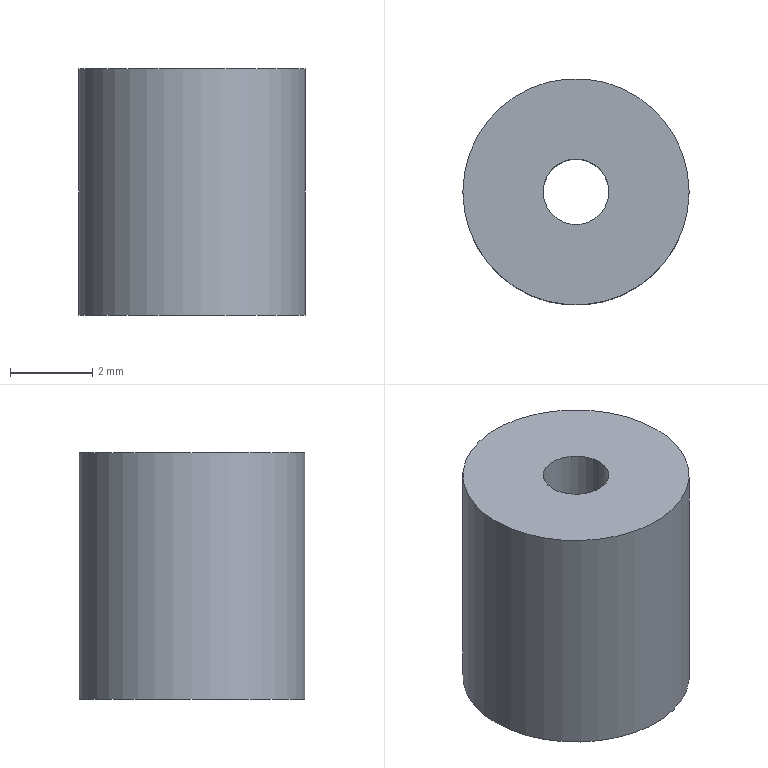Part | STEP file | Radial combiner dielectric | 1 solid | 4 faces | box 5.5 x 5.5 x 6 mm | volume 130.486 mm3 | cylinder 2 | plane 2 | commonest cylinder face diameters 1.6 x1 5.5 x1
STEP:
#1=CARTESIAN_POINT('',(0.,0.,0.));
#2=DIRECTION('',(0.,0.,1.));
#3=DIRECTION('',(1.,0.,0.));
#4=AXIS2_PLACEMENT_3D('',#1,#2,#3);
#5=CARTESIAN_POINT('',(-195.141,-219.765,70.172));
#6=VERTEX_POINT('',#5);
#7=CARTESIAN_POINT('',(-192.391,-219.765,70.172));
#8=DIRECTION('',(0.,0.,-1.));
#9=DIRECTION('',(-1.,0.,0.));
#10=AXIS2_PLACEMENT_3D('',#7,#8,#9);
#11=CIRCLE('',#10,2.75);
#12=CARTESIAN_POINT('',(-192.391,-219.765,70.172));
#13=DIRECTION('',(0.,0.,-1.));
#14=DIRECTION('',(-1.,0.,0.));
#15=AXIS2_PLACEMENT_3D('',#12,#13,#14);
#16=CYLINDRICAL_SURFACE('',#15,2.75);
#17=CARTESIAN_POINT('',(0.,0.));
#18=DIRECTION('',(1.,0.));
#19=VECTOR('',#18,1.);
#20=LINE('',#17,#19);
#21=(GEOMETRIC_REPRESENTATION_CONTEXT(2)PARAMETRIC_REPRESENTATION_CONTEXT()REPRESENTATION_CONTEXT('',''));
#22=DEFINITIONAL_REPRESENTATION('',(#20),#21);
#23=PCURVE('',#16,#22);
#24=CARTESIAN_POINT('',(-192.391,-219.765,70.172));
#25=DIRECTION('',(0.,0.,-1.));
#26=DIRECTION('',(-1.,0.,0.));
#27=AXIS2_PLACEMENT_3D('',#24,#25,#26);
#28=PLANE('',#27);
#29=CARTESIAN_POINT('',(0.,0.));
#30=DIRECTION('',(1.,0.));
#31=AXIS2_PLACEMENT_2D('',#29,#30);
#32=CIRCLE('',#31,2.75);
#33=(GEOMETRIC_REPRESENTATION_CONTEXT(2)PARAMETRIC_REPRESENTATION_CONTEXT()REPRESENTATION_CONTEXT('',''));
#34=DEFINITIONAL_REPRESENTATION('',(#32),#33);
#35=PCURVE('',#28,#34);
#36=SURFACE_CURVE('',#11,(#23,#35),.PCURVE_S1.);
#37=EDGE_CURVE('',#6,#6,#36,.T.);
#38=ORIENTED_EDGE('',*,*,#37,.T.);
#39=CARTESIAN_POINT('',(-195.141,-219.765,64.172));
#40=VERTEX_POINT('',#39);
#41=CARTESIAN_POINT('',(-195.141,-219.765,70.172));
#42=CARTESIAN_POINT('',(-195.141,-219.765,64.172));
#43=B_SPLINE_CURVE_WITH_KNOTS('',1,(#41,#42),.UNSPECIFIED.,.F.,.F.,(2,2),(0.,6.),.PIECEWISE_BEZIER_KNOTS.);
#44=CARTESIAN_POINT('',(6.283,0.));
#45=DIRECTION('',(0.,1.));
#46=VECTOR('',#45,1.);
#47=LINE('',#44,#46);
#48=(GEOMETRIC_REPRESENTATION_CONTEXT(2)PARAMETRIC_REPRESENTATION_CONTEXT()REPRESENTATION_CONTEXT('',''));
#49=DEFINITIONAL_REPRESENTATION('',(#47),#48);
#50=PCURVE('',#16,#49);
#51=CARTESIAN_POINT('',(0.,0.));
#52=DIRECTION('',(0.,1.));
#53=VECTOR('',#52,1.);
#54=LINE('',#51,#53);
#55=(GEOMETRIC_REPRESENTATION_CONTEXT(2)PARAMETRIC_REPRESENTATION_CONTEXT()REPRESENTATION_CONTEXT('',''));
#56=DEFINITIONAL_REPRESENTATION('',(#54),#55);
#57=PCURVE('',#16,#56);
#58=SEAM_CURVE('',#43,(#50,#57),.PCURVE_S1.);
#59=EDGE_CURVE('',#6,#40,#58,.T.);
#60=ORIENTED_EDGE('',*,*,#59,.T.);
#61=CARTESIAN_POINT('',(-192.391,-219.765,64.172));
#62=DIRECTION('',(0.,0.,-1.));
#63=DIRECTION('',(-1.,0.,0.));
#64=AXIS2_PLACEMENT_3D('',#61,#62,#63);
#65=CIRCLE('',#64,2.75);
#66=CARTESIAN_POINT('',(0.,6.));
#67=DIRECTION('',(1.,0.));
#68=VECTOR('',#67,1.);
#69=LINE('',#66,#68);
#70=(GEOMETRIC_REPRESENTATION_CONTEXT(2)PARAMETRIC_REPRESENTATION_CONTEXT()REPRESENTATION_CONTEXT('',''));
#71=DEFINITIONAL_REPRESENTATION('',(#69),#70);
#72=PCURVE('',#16,#71);
#73=CARTESIAN_POINT('',(-192.391,-219.765,64.172));
#74=DIRECTION('',(0.,0.,-1.));
#75=DIRECTION('',(-1.,0.,0.));
#76=AXIS2_PLACEMENT_3D('',#73,#74,#75);
#77=PLANE('',#76);
#78=CARTESIAN_POINT('',(0.,0.));
#79=DIRECTION('',(1.,0.));
#80=AXIS2_PLACEMENT_2D('',#78,#79);
#81=CIRCLE('',#80,2.75);
#82=(GEOMETRIC_REPRESENTATION_CONTEXT(2)PARAMETRIC_REPRESENTATION_CONTEXT()REPRESENTATION_CONTEXT('',''));
#83=DEFINITIONAL_REPRESENTATION('',(#81),#82);
#84=PCURVE('',#77,#83);
#85=SURFACE_CURVE('',#65,(#72,#84),.PCURVE_S1.);
#86=EDGE_CURVE('',#40,#40,#85,.T.);
#87=ORIENTED_EDGE('',*,*,#86,.F.);
#88=ORIENTED_EDGE('',*,*,#59,.F.);
#89=EDGE_LOOP('',(#38,#60,#87,#88));
#90=FACE_BOUND('',#89,.T.);
#91=ADVANCED_FACE('',(#90),#16,.T.);
#92=CARTESIAN_POINT('',(-193.191,-219.765,70.172));
#93=VERTEX_POINT('',#92);
#94=CARTESIAN_POINT('',(-192.391,-219.765,70.172));
#95=DIRECTION('',(0.,0.,-1.));
#96=DIRECTION('',(-1.,0.,0.));
#97=AXIS2_PLACEMENT_3D('',#94,#95,#96);
#98=CIRCLE('',#97,0.8);
#99=CARTESIAN_POINT('',(0.,0.));
#100=DIRECTION('',(1.,0.));
#101=AXIS2_PLACEMENT_2D('',#99,#100);
#102=CIRCLE('',#101,0.8);
#103=(GEOMETRIC_REPRESENTATION_CONTEXT(2)PARAMETRIC_REPRESENTATION_CONTEXT()REPRESENTATION_CONTEXT('',''));
#104=DEFINITIONAL_REPRESENTATION('',(#102),#103);
#105=PCURVE('',#28,#104);
#106=CARTESIAN_POINT('',(-192.391,-219.765,70.172));
#107=DIRECTION('',(0.,0.,-1.));
#108=DIRECTION('',(-1.,0.,0.));
#109=AXIS2_PLACEMENT_3D('',#106,#107,#108);
#110=CYLINDRICAL_SURFACE('',#109,0.8);
#111=CARTESIAN_POINT('',(0.,0.));
#112=DIRECTION('',(1.,0.));
#113=VECTOR('',#112,1.);
#114=LINE('',#111,#113);
#115=(GEOMETRIC_REPRESENTATION_CONTEXT(2)PARAMETRIC_REPRESENTATION_CONTEXT()REPRESENTATION_CONTEXT('',''));
#116=DEFINITIONAL_REPRESENTATION('',(#114),#115);
#117=PCURVE('',#110,#116);
#118=SURFACE_CURVE('',#98,(#105,#117),.PCURVE_S1.);
#119=EDGE_CURVE('',#93,#93,#118,.T.);
#120=ORIENTED_EDGE('',*,*,#119,.T.);
#121=EDGE_LOOP('',(#120));
#122=FACE_BOUND('',#121,.T.);
#123=ORIENTED_EDGE('',*,*,#37,.F.);
#124=EDGE_LOOP('',(#123));
#125=FACE_BOUND('',#124,.T.);
#126=ADVANCED_FACE('',(#122,#125),#28,.F.);
#127=CARTESIAN_POINT('',(-193.191,-219.765,64.172));
#128=VERTEX_POINT('',#127);
#129=CARTESIAN_POINT('',(-192.391,-219.765,64.172));
#130=DIRECTION('',(0.,0.,-1.));
#131=DIRECTION('',(-1.,0.,0.));
#132=AXIS2_PLACEMENT_3D('',#129,#130,#131);
#133=CIRCLE('',#132,0.8);
#134=CARTESIAN_POINT('',(0.,0.));
#135=DIRECTION('',(1.,0.));
#136=AXIS2_PLACEMENT_2D('',#134,#135);
#137=CIRCLE('',#136,0.8);
#138=(GEOMETRIC_REPRESENTATION_CONTEXT(2)PARAMETRIC_REPRESENTATION_CONTEXT()REPRESENTATION_CONTEXT('',''));
#139=DEFINITIONAL_REPRESENTATION('',(#137),#138);
#140=PCURVE('',#77,#139);
#141=CARTESIAN_POINT('',(0.,6.));
#142=DIRECTION('',(1.,0.));
#143=VECTOR('',#142,1.);
#144=LINE('',#141,#143);
#145=(GEOMETRIC_REPRESENTATION_CONTEXT(2)PARAMETRIC_REPRESENTATION_CONTEXT()REPRESENTATION_CONTEXT('',''));
#146=DEFINITIONAL_REPRESENTATION('',(#144),#145);
#147=PCURVE('',#110,#146);
#148=SURFACE_CURVE('',#133,(#140,#147),.PCURVE_S1.);
#149=EDGE_CURVE('',#128,#128,#148,.T.);
#150=ORIENTED_EDGE('',*,*,#149,.F.);
#151=EDGE_LOOP('',(#150));
#152=FACE_BOUND('',#151,.T.);
#153=ORIENTED_EDGE('',*,*,#86,.T.);
#154=EDGE_LOOP('',(#153));
#155=FACE_BOUND('',#154,.T.);
#156=ADVANCED_FACE('',(#152,#155),#77,.T.);
#157=ORIENTED_EDGE('',*,*,#149,.F.);
#158=CARTESIAN_POINT('',(-193.191,-219.765,70.172));
#159=CARTESIAN_POINT('',(-193.191,-219.765,64.172));
#160=B_SPLINE_CURVE_WITH_KNOTS('',1,(#158,#159),.UNSPECIFIED.,.F.,.F.,(2,2),(0.,6.),.PIECEWISE_BEZIER_KNOTS.);
#161=CARTESIAN_POINT('',(0.,0.));
#162=DIRECTION('',(0.,1.));
#163=VECTOR('',#162,1.);
#164=LINE('',#161,#163);
#165=(GEOMETRIC_REPRESENTATION_CONTEXT(2)PARAMETRIC_REPRESENTATION_CONTEXT()REPRESENTATION_CONTEXT('',''));
#166=DEFINITIONAL_REPRESENTATION('',(#164),#165);
#167=PCURVE('',#110,#166);
#168=CARTESIAN_POINT('',(6.283,0.));
#169=DIRECTION('',(0.,1.));
#170=VECTOR('',#169,1.);
#171=LINE('',#168,#170);
#172=(GEOMETRIC_REPRESENTATION_CONTEXT(2)PARAMETRIC_REPRESENTATION_CONTEXT()REPRESENTATION_CONTEXT('',''));
#173=DEFINITIONAL_REPRESENTATION('',(#171),#172);
#174=PCURVE('',#110,#173);
#175=SEAM_CURVE('',#160,(#167,#174),.PCURVE_S1.);
#176=EDGE_CURVE('',#93,#128,#175,.T.);
#177=ORIENTED_EDGE('',*,*,#176,.F.);
#178=ORIENTED_EDGE('',*,*,#119,.T.);
#179=ORIENTED_EDGE('',*,*,#176,.T.);
#180=EDGE_LOOP('',(#157,#177,#178,#179));
#181=FACE_BOUND('',#180,.F.);
#182=ADVANCED_FACE('',(#181),#110,.F.);
#183=CLOSED_SHELL('',(#91,#126,#156,#182));
#184=MANIFOLD_SOLID_BREP('',#183);
#185=(LENGTH_UNIT()NAMED_UNIT(*)SI_UNIT(.MILLI.,.METRE.));
#186=UNCERTAINTY_MEASURE_WITH_UNIT(LENGTH_MEASURE(0.00001),#185,'','');
#187=(NAMED_UNIT(*)PLANE_ANGLE_UNIT()SI_UNIT($,.RADIAN.));
#188=(NAMED_UNIT(*)SI_UNIT($,.STERADIAN.)SOLID_ANGLE_UNIT());
#189=(GEOMETRIC_REPRESENTATION_CONTEXT(3)GLOBAL_UNCERTAINTY_ASSIGNED_CONTEXT((#186))GLOBAL_UNIT_ASSIGNED_CONTEXT((#185,#187,#188))REPRESENTATION_CONTEXT('',''));
#190=ADVANCED_BREP_SHAPE_REPRESENTATION('',(#4,#184),#189);